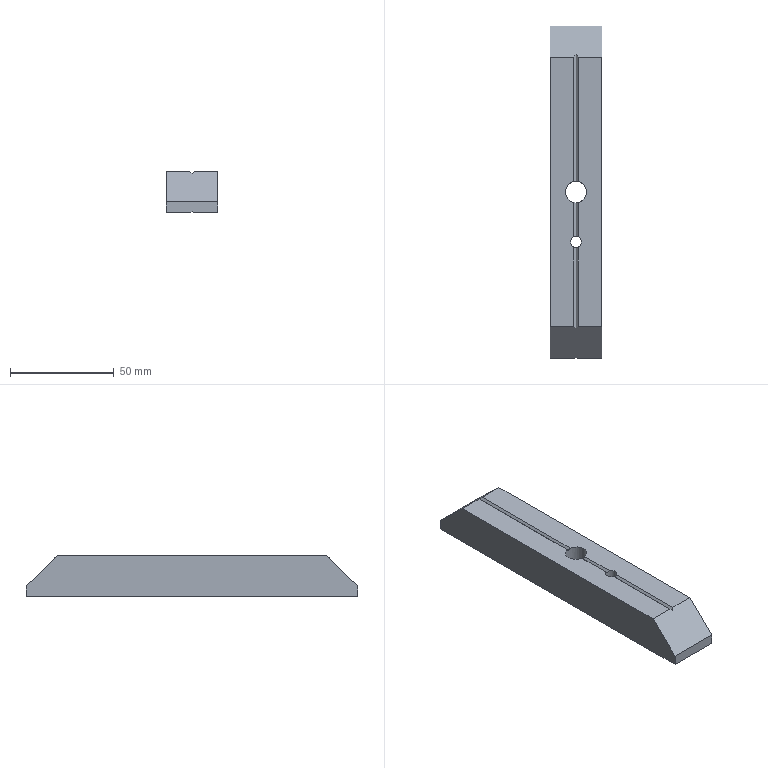Part | NX | features EXTRUDE 3, DATUM_CSYS 1 | 1 solid | 25 faces | box 25 x 160 x 19.5 mm | volume 70356 mm3 | plane 22 | cylinder 2 | spline 1 | commonest cylinder face diameters 5.3 x1 10.3 x1
STEP:
#1=CARTESIAN_POINT('',(3903.536,6799.606,-19.5));
#2=VERTEX_POINT('',#1);
#3=CARTESIAN_POINT('',(3915.536,6799.606,-19.5));
#4=VERTEX_POINT('',#3);
#5=CARTESIAN_POINT('',(3890.536,6799.606,-19.5));
#6=DIRECTION('',(1.,0.,0.));
#7=VECTOR('',#6,1000.);
#8=LINE('',#5,#7);
#9=EDGE_CURVE('',#2,#4,#8,.T.);
#10=ORIENTED_EDGE('',*,*,#9,.F.);
#11=CARTESIAN_POINT('',(3903.536,6853.003,-19.5));
#12=VERTEX_POINT('',#11);
#13=CARTESIAN_POINT('',(3903.536,6978.016,-19.5));
#14=DIRECTION('',(0.,-1.,0.));
#15=VECTOR('',#14,1000.);
#16=LINE('',#13,#15);
#17=EDGE_CURVE('',#2,#12,#16,.F.);
#18=ORIENTED_EDGE('',*,*,#17,.T.);
#19=CARTESIAN_POINT('',(3903.536,6858.208,-19.5));
#20=VERTEX_POINT('',#19);
#21=CARTESIAN_POINT('',(3903.036,6855.606,-19.5));
#22=DIRECTION('',(0.,0.,1.));
#23=DIRECTION('',(1.,0.,0.));
#24=AXIS2_PLACEMENT_3D('',#21,#22,#23);
#25=CIRCLE('',#24,2.65);
#26=EDGE_CURVE('',#12,#20,#25,.T.);
#27=ORIENTED_EDGE('',*,*,#26,.T.);
#28=CARTESIAN_POINT('',(3903.536,6874.48,-19.5));
#29=VERTEX_POINT('',#28);
#30=CARTESIAN_POINT('',(3903.536,6978.016,-19.5));
#31=DIRECTION('',(0.,-1.,0.));
#32=VECTOR('',#31,1000.);
#33=LINE('',#30,#32);
#34=EDGE_CURVE('',#20,#29,#33,.F.);
#35=ORIENTED_EDGE('',*,*,#34,.T.);
#36=CARTESIAN_POINT('',(3903.536,6884.731,-19.5));
#37=VERTEX_POINT('',#36);
#38=CARTESIAN_POINT('',(3903.036,6879.606,-19.5));
#39=DIRECTION('',(0.,0.,1.));
#40=DIRECTION('',(1.,0.,0.));
#41=AXIS2_PLACEMENT_3D('',#38,#39,#40);
#42=CIRCLE('',#41,5.15);
#43=EDGE_CURVE('',#29,#37,#42,.T.);
#44=ORIENTED_EDGE('',*,*,#43,.T.);
#45=CARTESIAN_POINT('',(3903.536,6959.606,-19.5));
#46=VERTEX_POINT('',#45);
#47=CARTESIAN_POINT('',(3903.536,6978.016,-19.5));
#48=DIRECTION('',(0.,-1.,0.));
#49=VECTOR('',#48,1000.);
#50=LINE('',#47,#49);
#51=EDGE_CURVE('',#37,#46,#50,.F.);
#52=ORIENTED_EDGE('',*,*,#51,.T.);
#53=CARTESIAN_POINT('',(3915.536,6959.606,-19.5));
#54=VERTEX_POINT('',#53);
#55=CARTESIAN_POINT('',(3890.536,6959.606,-19.5));
#56=DIRECTION('',(1.,0.,0.));
#57=VECTOR('',#56,1000.);
#58=LINE('',#55,#57);
#59=EDGE_CURVE('',#46,#54,#58,.T.);
#60=ORIENTED_EDGE('',*,*,#59,.T.);
#61=CARTESIAN_POINT('',(3915.536,6959.606,-19.5));
#62=DIRECTION('',(0.,-1.,0.));
#63=VECTOR('',#62,1000.);
#64=LINE('',#61,#63);
#65=EDGE_CURVE('',#54,#4,#64,.T.);
#66=ORIENTED_EDGE('',*,*,#65,.T.);
#67=EDGE_LOOP('',(#10,#18,#27,#35,#44,#52,#60,#66));
#68=FACE_BOUND('',#67,.T.);
#69=CARTESIAN_POINT('',(3890.536,6959.606,-19.5));
#70=DIRECTION('',(0.,0.,1.));
#71=DIRECTION('',(1.,0.,0.));
#72=AXIS2_PLACEMENT_3D('',#69,#70,#71);
#73=PLANE('',#72);
#74=ADVANCED_FACE('',(#68),#73,.F.);
#75=CARTESIAN_POINT('',(3902.536,6858.208,-19.5));
#76=VERTEX_POINT('',#75);
#77=CARTESIAN_POINT('',(3902.536,6853.003,-19.5));
#78=VERTEX_POINT('',#77);
#79=CARTESIAN_POINT('',(3903.036,6855.606,-19.5));
#80=DIRECTION('',(0.,0.,1.));
#81=DIRECTION('',(1.,0.,0.));
#82=AXIS2_PLACEMENT_3D('',#79,#80,#81);
#83=CIRCLE('',#82,2.65);
#84=EDGE_CURVE('',#76,#78,#83,.T.);
#85=ORIENTED_EDGE('',*,*,#84,.T.);
#86=CARTESIAN_POINT('',(3902.536,6799.606,-19.5));
#87=VERTEX_POINT('',#86);
#88=CARTESIAN_POINT('',(3902.536,6978.016,-19.5));
#89=DIRECTION('',(0.,1.,0.));
#90=VECTOR('',#89,1000.);
#91=LINE('',#88,#90);
#92=EDGE_CURVE('',#78,#87,#91,.F.);
#93=ORIENTED_EDGE('',*,*,#92,.T.);
#94=CARTESIAN_POINT('',(3890.536,6799.606,-19.5));
#95=VERTEX_POINT('',#94);
#96=CARTESIAN_POINT('',(3890.536,6799.606,-19.5));
#97=DIRECTION('',(1.,0.,0.));
#98=VECTOR('',#97,1000.);
#99=LINE('',#96,#98);
#100=EDGE_CURVE('',#95,#87,#99,.T.);
#101=ORIENTED_EDGE('',*,*,#100,.F.);
#102=CARTESIAN_POINT('',(3890.536,6959.606,-19.5));
#103=VERTEX_POINT('',#102);
#104=CARTESIAN_POINT('',(3890.536,6959.606,-19.5));
#105=DIRECTION('',(0.,-1.,0.));
#106=VECTOR('',#105,1000.);
#107=LINE('',#104,#106);
#108=EDGE_CURVE('',#103,#95,#107,.T.);
#109=ORIENTED_EDGE('',*,*,#108,.F.);
#110=CARTESIAN_POINT('',(3902.536,6959.606,-19.5));
#111=VERTEX_POINT('',#110);
#112=CARTESIAN_POINT('',(3890.536,6959.606,-19.5));
#113=DIRECTION('',(1.,0.,0.));
#114=VECTOR('',#113,1000.);
#115=LINE('',#112,#114);
#116=EDGE_CURVE('',#103,#111,#115,.T.);
#117=ORIENTED_EDGE('',*,*,#116,.T.);
#118=CARTESIAN_POINT('',(3902.536,6884.731,-19.5));
#119=VERTEX_POINT('',#118);
#120=CARTESIAN_POINT('',(3902.536,6978.016,-19.5));
#121=DIRECTION('',(0.,1.,0.));
#122=VECTOR('',#121,1000.);
#123=LINE('',#120,#122);
#124=EDGE_CURVE('',#111,#119,#123,.F.);
#125=ORIENTED_EDGE('',*,*,#124,.T.);
#126=CARTESIAN_POINT('',(3902.036,6874.554,-19.5));
#127=VERTEX_POINT('',#126);
#128=CARTESIAN_POINT('',(3903.036,6879.606,-19.5));
#129=DIRECTION('',(0.,0.,1.));
#130=DIRECTION('',(1.,0.,0.));
#131=AXIS2_PLACEMENT_3D('',#128,#129,#130);
#132=CIRCLE('',#131,5.15);
#133=EDGE_CURVE('',#119,#127,#132,.T.);
#134=ORIENTED_EDGE('',*,*,#133,.T.);
#135=CARTESIAN_POINT('',(3902.536,6874.48,-19.5));
#136=VERTEX_POINT('',#135);
#137=CARTESIAN_POINT('',(3903.036,6879.606,-19.5));
#138=DIRECTION('',(0.,0.,-1.));
#139=DIRECTION('',(-0.9963,0.0857,0.));
#140=AXIS2_PLACEMENT_3D('',#137,#138,#139);
#141=ELLIPSE('',#140,5.15,5.15);
#142=EDGE_CURVE('',#127,#136,#141,.F.);
#143=ORIENTED_EDGE('',*,*,#142,.T.);
#144=CARTESIAN_POINT('',(3902.536,6978.016,-19.5));
#145=DIRECTION('',(0.,1.,0.));
#146=VECTOR('',#145,1000.);
#147=LINE('',#144,#146);
#148=EDGE_CURVE('',#136,#76,#147,.F.);
#149=ORIENTED_EDGE('',*,*,#148,.T.);
#150=EDGE_LOOP('',(#85,#93,#101,#109,#117,#125,#134,#143,#149));
#151=FACE_BOUND('',#150,.T.);
#152=CARTESIAN_POINT('',(3890.536,6959.606,-19.5));
#153=DIRECTION('',(0.,0.,1.));
#154=DIRECTION('',(1.,0.,0.));
#155=AXIS2_PLACEMENT_3D('',#152,#153,#154);
#156=PLANE('',#155);
#157=ADVANCED_FACE('',(#151),#156,.F.);
#158=CARTESIAN_POINT('',(3904.036,6858.06,0.));
#159=VERTEX_POINT('',#158);
#160=CARTESIAN_POINT('',(3904.036,6853.151,0.));
#161=VERTEX_POINT('',#160);
#162=CARTESIAN_POINT('',(3903.036,6855.606,0.));
#163=DIRECTION('',(0.,0.,-1.));
#164=DIRECTION('',(1.,0.,0.));
#165=AXIS2_PLACEMENT_3D('',#162,#163,#164);
#166=CIRCLE('',#165,2.65);
#167=EDGE_CURVE('',#159,#161,#166,.T.);
#168=ORIENTED_EDGE('',*,*,#167,.T.);
#169=CARTESIAN_POINT('',(3904.036,6814.606,0.));
#170=VERTEX_POINT('',#169);
#171=CARTESIAN_POINT('',(3904.036,6978.016,0.));
#172=DIRECTION('',(0.,1.,0.));
#173=VECTOR('',#172,1000.);
#174=LINE('',#171,#173);
#175=EDGE_CURVE('',#161,#170,#174,.F.);
#176=ORIENTED_EDGE('',*,*,#175,.T.);
#177=CARTESIAN_POINT('',(3915.536,6814.606,0.));
#178=VERTEX_POINT('',#177);
#179=CARTESIAN_POINT('',(3890.536,6814.606,0.));
#180=DIRECTION('',(1.,0.,0.));
#181=VECTOR('',#180,1000.);
#182=LINE('',#179,#181);
#183=EDGE_CURVE('',#170,#178,#182,.T.);
#184=ORIENTED_EDGE('',*,*,#183,.T.);
#185=CARTESIAN_POINT('',(3915.536,6944.606,0.));
#186=VERTEX_POINT('',#185);
#187=CARTESIAN_POINT('',(3915.536,6814.606,0.));
#188=DIRECTION('',(0.,1.,0.));
#189=VECTOR('',#188,1000.);
#190=LINE('',#187,#189);
#191=EDGE_CURVE('',#178,#186,#190,.T.);
#192=ORIENTED_EDGE('',*,*,#191,.T.);
#193=CARTESIAN_POINT('',(3904.036,6944.606,0.));
#194=VERTEX_POINT('',#193);
#195=CARTESIAN_POINT('',(3890.536,6944.606,0.));
#196=DIRECTION('',(1.,0.,0.));
#197=VECTOR('',#196,1000.);
#198=LINE('',#195,#197);
#199=EDGE_CURVE('',#194,#186,#198,.T.);
#200=ORIENTED_EDGE('',*,*,#199,.F.);
#201=CARTESIAN_POINT('',(3904.036,6884.657,0.));
#202=VERTEX_POINT('',#201);
#203=CARTESIAN_POINT('',(3904.036,6978.016,0.));
#204=DIRECTION('',(0.,1.,0.));
#205=VECTOR('',#204,1000.);
#206=LINE('',#203,#205);
#207=EDGE_CURVE('',#194,#202,#206,.F.);
#208=ORIENTED_EDGE('',*,*,#207,.T.);
#209=CARTESIAN_POINT('',(3904.036,6874.554,0.));
#210=VERTEX_POINT('',#209);
#211=CARTESIAN_POINT('',(3903.036,6879.606,0.));
#212=DIRECTION('',(0.,0.,-1.));
#213=DIRECTION('',(1.,0.,0.));
#214=AXIS2_PLACEMENT_3D('',#211,#212,#213);
#215=CIRCLE('',#214,5.15);
#216=EDGE_CURVE('',#202,#210,#215,.T.);
#217=ORIENTED_EDGE('',*,*,#216,.T.);
#218=CARTESIAN_POINT('',(3904.036,6978.016,0.));
#219=DIRECTION('',(0.,1.,0.));
#220=VECTOR('',#219,1000.);
#221=LINE('',#218,#220);
#222=EDGE_CURVE('',#210,#159,#221,.F.);
#223=ORIENTED_EDGE('',*,*,#222,.T.);
#224=EDGE_LOOP('',(#168,#176,#184,#192,#200,#208,#217,#223));
#225=FACE_BOUND('',#224,.T.);
#226=CARTESIAN_POINT('',(3890.536,6814.606,0.));
#227=DIRECTION('',(0.,0.,-1.));
#228=DIRECTION('',(0.,1.,0.));
#229=AXIS2_PLACEMENT_3D('',#226,#227,#228);
#230=PLANE('',#229);
#231=ADVANCED_FACE('',(#225),#230,.F.);
#232=CARTESIAN_POINT('',(3890.536,6814.606,0.));
#233=VERTEX_POINT('',#232);
#234=CARTESIAN_POINT('',(3902.036,6814.606,0.));
#235=VERTEX_POINT('',#234);
#236=CARTESIAN_POINT('',(3890.536,6814.606,0.));
#237=DIRECTION('',(1.,0.,0.));
#238=VECTOR('',#237,1000.);
#239=LINE('',#236,#238);
#240=EDGE_CURVE('',#233,#235,#239,.T.);
#241=ORIENTED_EDGE('',*,*,#240,.T.);
#242=CARTESIAN_POINT('',(3902.036,6853.151,0.));
#243=VERTEX_POINT('',#242);
#244=CARTESIAN_POINT('',(3902.036,6978.016,0.));
#245=DIRECTION('',(0.,-1.,0.));
#246=VECTOR('',#245,1000.);
#247=LINE('',#244,#246);
#248=EDGE_CURVE('',#235,#243,#247,.F.);
#249=ORIENTED_EDGE('',*,*,#248,.T.);
#250=CARTESIAN_POINT('',(3902.036,6858.06,0.));
#251=VERTEX_POINT('',#250);
#252=CARTESIAN_POINT('',(3903.036,6855.606,0.));
#253=DIRECTION('',(0.,0.,-1.));
#254=DIRECTION('',(1.,0.,0.));
#255=AXIS2_PLACEMENT_3D('',#252,#253,#254);
#256=CIRCLE('',#255,2.65);
#257=EDGE_CURVE('',#243,#251,#256,.T.);
#258=ORIENTED_EDGE('',*,*,#257,.T.);
#259=CARTESIAN_POINT('',(3902.036,6874.554,0.));
#260=VERTEX_POINT('',#259);
#261=CARTESIAN_POINT('',(3902.036,6978.016,0.));
#262=DIRECTION('',(0.,-1.,0.));
#263=VECTOR('',#262,1000.);
#264=LINE('',#261,#263);
#265=EDGE_CURVE('',#251,#260,#264,.F.);
#266=ORIENTED_EDGE('',*,*,#265,.T.);
#267=CARTESIAN_POINT('',(3902.036,6884.657,0.));
#268=VERTEX_POINT('',#267);
#269=CARTESIAN_POINT('',(3903.036,6879.606,0.));
#270=DIRECTION('',(0.,0.,-1.));
#271=DIRECTION('',(1.,0.,0.));
#272=AXIS2_PLACEMENT_3D('',#269,#270,#271);
#273=CIRCLE('',#272,5.15);
#274=EDGE_CURVE('',#260,#268,#273,.T.);
#275=ORIENTED_EDGE('',*,*,#274,.T.);
#276=CARTESIAN_POINT('',(3902.036,6944.606,0.));
#277=VERTEX_POINT('',#276);
#278=CARTESIAN_POINT('',(3902.036,6978.016,0.));
#279=DIRECTION('',(0.,-1.,0.));
#280=VECTOR('',#279,1000.);
#281=LINE('',#278,#280);
#282=EDGE_CURVE('',#268,#277,#281,.F.);
#283=ORIENTED_EDGE('',*,*,#282,.T.);
#284=CARTESIAN_POINT('',(3890.536,6944.606,0.));
#285=VERTEX_POINT('',#284);
#286=CARTESIAN_POINT('',(3890.536,6944.606,0.));
#287=DIRECTION('',(1.,0.,0.));
#288=VECTOR('',#287,1000.);
#289=LINE('',#286,#288);
#290=EDGE_CURVE('',#285,#277,#289,.T.);
#291=ORIENTED_EDGE('',*,*,#290,.F.);
#292=CARTESIAN_POINT('',(3890.536,6814.606,0.));
#293=DIRECTION('',(0.,1.,0.));
#294=VECTOR('',#293,1000.);
#295=LINE('',#292,#294);
#296=EDGE_CURVE('',#233,#285,#295,.T.);
#297=ORIENTED_EDGE('',*,*,#296,.F.);
#298=EDGE_LOOP('',(#241,#249,#258,#266,#275,#283,#291,#297));
#299=FACE_BOUND('',#298,.T.);
#300=CARTESIAN_POINT('',(3890.536,6814.606,0.));
#301=DIRECTION('',(0.,0.,-1.));
#302=DIRECTION('',(0.,1.,0.));
#303=AXIS2_PLACEMENT_3D('',#300,#301,#302);
#304=PLANE('',#303);
#305=ADVANCED_FACE('',(#299),#304,.F.);
#306=CARTESIAN_POINT('',(3903.036,6884.756,-1.));
#307=VERTEX_POINT('',#306);
#308=CARTESIAN_POINT('',(3903.036,6879.606,-1.));
#309=DIRECTION('',(0.7071,0.,-0.7071));
#310=DIRECTION('',(0.7071,0.,0.7071));
#311=AXIS2_PLACEMENT_3D('',#308,#309,#310);
#312=ELLIPSE('',#311,7.283,5.15);
#313=EDGE_CURVE('',#202,#307,#312,.F.);
#314=ORIENTED_EDGE('',*,*,#313,.T.);
#315=CARTESIAN_POINT('',(3903.036,6879.606,-1.));
#316=DIRECTION('',(-0.7071,0.,-0.7071));
#317=DIRECTION('',(-0.7071,0.,0.7071));
#318=AXIS2_PLACEMENT_3D('',#315,#316,#317);
#319=ELLIPSE('',#318,7.283,5.15);
#320=EDGE_CURVE('',#307,#268,#319,.F.);
#321=ORIENTED_EDGE('',*,*,#320,.T.);
#322=ORIENTED_EDGE('',*,*,#274,.F.);
#323=CARTESIAN_POINT('',(3902.036,6874.554,-19.5));
#324=CARTESIAN_POINT('',(3902.036,6874.554,-13.));
#325=CARTESIAN_POINT('',(3902.036,6874.554,-6.5));
#326=CARTESIAN_POINT('',(3902.036,6874.554,0.));
#327=B_SPLINE_CURVE_WITH_KNOTS('',3,(#323,#324,#325,#326),.UNSPECIFIED.,.F.,.F.,(4,4),(0.9996,1.),.UNSPECIFIED.);
#328=EDGE_CURVE('',#127,#260,#327,.T.);
#329=ORIENTED_EDGE('',*,*,#328,.F.);
#330=ORIENTED_EDGE('',*,*,#133,.F.);
#331=CARTESIAN_POINT('',(3903.036,6884.756,-19.));
#332=VERTEX_POINT('',#331);
#333=CARTESIAN_POINT('',(3903.036,6879.606,-19.));
#334=DIRECTION('',(-0.7071,0.,0.7071));
#335=DIRECTION('',(0.7071,0.,0.7071));
#336=AXIS2_PLACEMENT_3D('',#333,#334,#335);
#337=ELLIPSE('',#336,7.283,5.15);
#338=EDGE_CURVE('',#119,#332,#337,.F.);
#339=ORIENTED_EDGE('',*,*,#338,.T.);
#340=CARTESIAN_POINT('',(3903.036,6879.606,-19.));
#341=DIRECTION('',(0.7071,0.,0.7071));
#342=DIRECTION('',(-0.7071,0.,0.7071));
#343=AXIS2_PLACEMENT_3D('',#340,#341,#342);
#344=ELLIPSE('',#343,7.283,5.15);
#345=EDGE_CURVE('',#332,#37,#344,.F.);
#346=ORIENTED_EDGE('',*,*,#345,.T.);
#347=ORIENTED_EDGE('',*,*,#43,.F.);
#348=CARTESIAN_POINT('',(3903.036,6874.456,-19.));
#349=VERTEX_POINT('',#348);
#350=CARTESIAN_POINT('',(3903.036,6879.606,-19.));
#351=DIRECTION('',(0.7071,0.,0.7071));
#352=DIRECTION('',(-0.7071,0.,0.7071));
#353=AXIS2_PLACEMENT_3D('',#350,#351,#352);
#354=ELLIPSE('',#353,7.283,5.15);
#355=EDGE_CURVE('',#29,#349,#354,.F.);
#356=ORIENTED_EDGE('',*,*,#355,.T.);
#357=CARTESIAN_POINT('',(3903.036,6874.456,-1.));
#358=VERTEX_POINT('',#357);
#359=CARTESIAN_POINT('',(3903.036,6874.456,-1.));
#360=CARTESIAN_POINT('',(3903.036,6874.456,-7.));
#361=CARTESIAN_POINT('',(3903.036,6874.456,-13.));
#362=CARTESIAN_POINT('',(3903.036,6874.456,-19.));
#363=B_SPLINE_CURVE_WITH_KNOTS('',3,(#359,#360,#361,#362),.UNSPECIFIED.,.F.,.F.,(4,4),(0.00001818,0.0003455),.UNSPECIFIED.);
#364=EDGE_CURVE('',#358,#349,#363,.T.);
#365=ORIENTED_EDGE('',*,*,#364,.F.);
#366=CARTESIAN_POINT('',(3903.036,6879.606,-1.));
#367=DIRECTION('',(0.7071,0.,-0.7071));
#368=DIRECTION('',(0.7071,0.,0.7071));
#369=AXIS2_PLACEMENT_3D('',#366,#367,#368);
#370=ELLIPSE('',#369,7.283,5.15);
#371=EDGE_CURVE('',#358,#210,#370,.F.);
#372=ORIENTED_EDGE('',*,*,#371,.T.);
#373=ORIENTED_EDGE('',*,*,#216,.F.);
#374=EDGE_LOOP('',(#314,#321,#322,#329,#330,#339,#346,#347,#356,#365,#372,#373));
#375=FACE_BOUND('',#374,.T.);
#376=CARTESIAN_POINT('',(3903.036,6879.606,-55000.));
#377=DIRECTION('',(0.,0.,1.));
#378=DIRECTION('',(1.,0.,0.));
#379=AXIS2_PLACEMENT_3D('',#376,#377,#378);
#380=CYLINDRICAL_SURFACE('',#379,5.15);
#381=ADVANCED_FACE('',(#375),#380,.F.);
#382=ORIENTED_EDGE('',*,*,#364,.T.);
#383=CARTESIAN_POINT('',(3903.036,6874.456,-19.));
#384=CARTESIAN_POINT('',(3902.869,6874.456,-19.167));
#385=CARTESIAN_POINT('',(3902.703,6874.464,-19.334));
#386=CARTESIAN_POINT('',(3902.536,6874.48,-19.5));
#387=B_SPLINE_CURVE_WITH_KNOTS('',3,(#383,#384,#385,#386),.UNSPECIFIED.,.F.,.F.,(4,4),(0.,0.0007075),.UNSPECIFIED.);
#388=EDGE_CURVE('',#349,#136,#387,.T.);
#389=ORIENTED_EDGE('',*,*,#388,.T.);
#390=ORIENTED_EDGE('',*,*,#142,.F.);
#391=ORIENTED_EDGE('',*,*,#328,.T.);
#392=CARTESIAN_POINT('',(3902.036,6874.554,-0.00001317));
#393=CARTESIAN_POINT('',(3902.368,6874.488,-0.3317));
#394=CARTESIAN_POINT('',(3902.701,6874.456,-0.6651));
#395=CARTESIAN_POINT('',(3903.036,6874.456,-1.));
#396=B_SPLINE_CURVE_WITH_KNOTS('',3,(#392,#393,#394,#395),.UNSPECIFIED.,.F.,.F.,(4,4),(0.,0.001418),.UNSPECIFIED.);
#397=EDGE_CURVE('',#260,#358,#396,.T.);
#398=ORIENTED_EDGE('',*,*,#397,.T.);
#399=EDGE_LOOP('',(#382,#389,#390,#391,#398));
#400=FACE_BOUND('',#399,.T.);
#401=CARTESIAN_POINT('',(3903.036,6874.456,-19.5));
#402=CARTESIAN_POINT('',(3903.036,6874.456,0.117));
#403=CARTESIAN_POINT('',(3902.701,6874.456,-19.5));
#404=CARTESIAN_POINT('',(3902.701,6874.456,0.117));
#405=CARTESIAN_POINT('',(3902.365,6874.488,-19.5));
#406=CARTESIAN_POINT('',(3902.365,6874.488,0.117));
#407=CARTESIAN_POINT('',(3902.036,6874.554,-19.5));
#408=CARTESIAN_POINT('',(3902.036,6874.554,0.117));
#409=B_SPLINE_SURFACE_WITH_KNOTS('',3,1,((#401,#402),(#403,#404),(#405,#406),(#407,#408)),.SURF_OF_LINEAR_EXTRUSION.,.F.,.F.,.F.,(4,4),(2,2),(4.627,4.822),(0.,1.),.PIECEWISE_BEZIER_KNOTS.);
#410=ADVANCED_FACE('',(#400),#409,.T.);
#411=ORIENTED_EDGE('',*,*,#26,.F.);
#412=CARTESIAN_POINT('',(3903.036,6852.956,-19.));
#413=VERTEX_POINT('',#412);
#414=CARTESIAN_POINT('',(3903.036,6855.606,-19.));
#415=DIRECTION('',(0.7071,0.,0.7071));
#416=DIRECTION('',(-0.7071,0.,0.7071));
#417=AXIS2_PLACEMENT_3D('',#414,#415,#416);
#418=ELLIPSE('',#417,3.748,2.65);
#419=EDGE_CURVE('',#12,#413,#418,.F.);
#420=ORIENTED_EDGE('',*,*,#419,.T.);
#421=CARTESIAN_POINT('',(3903.036,6855.606,-19.));
#422=DIRECTION('',(-0.7071,0.,0.7071));
#423=DIRECTION('',(0.7071,0.,0.7071));
#424=AXIS2_PLACEMENT_3D('',#421,#422,#423);
#425=ELLIPSE('',#424,3.748,2.65);
#426=EDGE_CURVE('',#413,#78,#425,.F.);
#427=ORIENTED_EDGE('',*,*,#426,.T.);
#428=ORIENTED_EDGE('',*,*,#84,.F.);
#429=CARTESIAN_POINT('',(3903.036,6858.256,-19.));
#430=VERTEX_POINT('',#429);
#431=CARTESIAN_POINT('',(3903.036,6855.606,-19.));
#432=DIRECTION('',(-0.7071,0.,0.7071));
#433=DIRECTION('',(0.7071,0.,0.7071));
#434=AXIS2_PLACEMENT_3D('',#431,#432,#433);
#435=ELLIPSE('',#434,3.748,2.65);
#436=EDGE_CURVE('',#76,#430,#435,.F.);
#437=ORIENTED_EDGE('',*,*,#436,.T.);
#438=CARTESIAN_POINT('',(3903.036,6855.606,-19.));
#439=DIRECTION('',(0.7071,0.,0.7071));
#440=DIRECTION('',(-0.7071,0.,0.7071));
#441=AXIS2_PLACEMENT_3D('',#438,#439,#440);
#442=ELLIPSE('',#441,3.748,2.65);
#443=EDGE_CURVE('',#430,#20,#442,.F.);
#444=ORIENTED_EDGE('',*,*,#443,.T.);
#445=EDGE_LOOP('',(#411,#420,#427,#428,#437,#444));
#446=FACE_BOUND('',#445,.T.);
#447=ORIENTED_EDGE('',*,*,#257,.F.);
#448=CARTESIAN_POINT('',(3903.036,6852.956,-1.));
#449=VERTEX_POINT('',#448);
#450=CARTESIAN_POINT('',(3903.036,6855.606,-1.));
#451=DIRECTION('',(-0.7071,0.,-0.7071));
#452=DIRECTION('',(-0.7071,0.,0.7071));
#453=AXIS2_PLACEMENT_3D('',#450,#451,#452);
#454=ELLIPSE('',#453,3.748,2.65);
#455=EDGE_CURVE('',#243,#449,#454,.F.);
#456=ORIENTED_EDGE('',*,*,#455,.T.);
#457=CARTESIAN_POINT('',(3903.036,6855.606,-1.));
#458=DIRECTION('',(0.7071,0.,-0.7071));
#459=DIRECTION('',(0.7071,0.,0.7071));
#460=AXIS2_PLACEMENT_3D('',#457,#458,#459);
#461=ELLIPSE('',#460,3.748,2.65);
#462=EDGE_CURVE('',#449,#161,#461,.F.);
#463=ORIENTED_EDGE('',*,*,#462,.T.);
#464=ORIENTED_EDGE('',*,*,#167,.F.);
#465=CARTESIAN_POINT('',(3903.036,6858.256,-1.));
#466=VERTEX_POINT('',#465);
#467=CARTESIAN_POINT('',(3903.036,6855.606,-1.));
#468=DIRECTION('',(0.7071,0.,-0.7071));
#469=DIRECTION('',(0.7071,0.,0.7071));
#470=AXIS2_PLACEMENT_3D('',#467,#468,#469);
#471=ELLIPSE('',#470,3.748,2.65);
#472=EDGE_CURVE('',#159,#466,#471,.F.);
#473=ORIENTED_EDGE('',*,*,#472,.T.);
#474=CARTESIAN_POINT('',(3903.036,6855.606,-1.));
#475=DIRECTION('',(-0.7071,0.,-0.7071));
#476=DIRECTION('',(-0.7071,0.,0.7071));
#477=AXIS2_PLACEMENT_3D('',#474,#475,#476);
#478=ELLIPSE('',#477,3.748,2.65);
#479=EDGE_CURVE('',#466,#251,#478,.F.);
#480=ORIENTED_EDGE('',*,*,#479,.T.);
#481=EDGE_LOOP('',(#447,#456,#463,#464,#473,#480));
#482=FACE_BOUND('',#481,.T.);
#483=CARTESIAN_POINT('',(3903.036,6855.606,-55000.));
#484=DIRECTION('',(0.,0.,1.));
#485=DIRECTION('',(1.,0.,0.));
#486=AXIS2_PLACEMENT_3D('',#483,#484,#485);
#487=CYLINDRICAL_SURFACE('',#486,2.65);
#488=ADVANCED_FACE('',(#446,#482),#487,.F.);
#489=CARTESIAN_POINT('',(3903.036,6959.606,-19.));
#490=VERTEX_POINT('',#489);
#491=CARTESIAN_POINT('',(3904.036,6959.606,-20.));
#492=DIRECTION('',(0.7071,0.,-0.7071));
#493=VECTOR('',#492,1000.);
#494=LINE('',#491,#493);
#495=EDGE_CURVE('',#46,#490,#494,.F.);
#496=ORIENTED_EDGE('',*,*,#495,.T.);
#497=CARTESIAN_POINT('',(3903.036,6959.606,-19.));
#498=DIRECTION('',(0.7071,0.,0.7071));
#499=VECTOR('',#498,1000.);
#500=LINE('',#497,#499);
#501=EDGE_CURVE('',#490,#111,#500,.F.);
#502=ORIENTED_EDGE('',*,*,#501,.T.);
#503=ORIENTED_EDGE('',*,*,#116,.F.);
#504=CARTESIAN_POINT('',(3890.536,6959.606,-14.5));
#505=VERTEX_POINT('',#504);
#506=CARTESIAN_POINT('',(3890.536,6959.606,-14.5));
#507=DIRECTION('',(0.,0.,-1.));
#508=VECTOR('',#507,1000.);
#509=LINE('',#506,#508);
#510=EDGE_CURVE('',#505,#103,#509,.T.);
#511=ORIENTED_EDGE('',*,*,#510,.F.);
#512=CARTESIAN_POINT('',(3915.536,6959.606,-14.5));
#513=VERTEX_POINT('',#512);
#514=CARTESIAN_POINT('',(3890.536,6959.606,-14.5));
#515=DIRECTION('',(1.,0.,0.));
#516=VECTOR('',#515,1000.);
#517=LINE('',#514,#516);
#518=EDGE_CURVE('',#505,#513,#517,.T.);
#519=ORIENTED_EDGE('',*,*,#518,.T.);
#520=CARTESIAN_POINT('',(3915.536,6959.606,-14.5));
#521=DIRECTION('',(0.,0.,-1.));
#522=VECTOR('',#521,1000.);
#523=LINE('',#520,#522);
#524=EDGE_CURVE('',#513,#54,#523,.T.);
#525=ORIENTED_EDGE('',*,*,#524,.T.);
#526=ORIENTED_EDGE('',*,*,#59,.F.);
#527=EDGE_LOOP('',(#496,#502,#503,#511,#519,#525,#526));
#528=FACE_BOUND('',#527,.T.);
#529=CARTESIAN_POINT('',(3890.536,6959.606,-14.5));
#530=DIRECTION('',(0.,-1.,0.));
#531=DIRECTION('',(0.,0.,-1.));
#532=AXIS2_PLACEMENT_3D('',#529,#530,#531);
#533=PLANE('',#532);
#534=ADVANCED_FACE('',(#528),#533,.F.);
#535=CARTESIAN_POINT('',(3903.036,6799.606,-19.));
#536=VERTEX_POINT('',#535);
#537=CARTESIAN_POINT('',(3903.036,6799.606,-19.));
#538=DIRECTION('',(-0.7071,0.,-0.7071));
#539=VECTOR('',#538,1000.);
#540=LINE('',#537,#539);
#541=EDGE_CURVE('',#87,#536,#540,.F.);
#542=ORIENTED_EDGE('',*,*,#541,.T.);
#543=CARTESIAN_POINT('',(3904.036,6799.606,-20.));
#544=DIRECTION('',(-0.7071,0.,0.7071));
#545=VECTOR('',#544,1000.);
#546=LINE('',#543,#545);
#547=EDGE_CURVE('',#536,#2,#546,.F.);
#548=ORIENTED_EDGE('',*,*,#547,.T.);
#549=ORIENTED_EDGE('',*,*,#9,.T.);
#550=CARTESIAN_POINT('',(3915.536,6799.606,-14.5));
#551=VERTEX_POINT('',#550);
#552=CARTESIAN_POINT('',(3915.536,6799.606,-19.5));
#553=DIRECTION('',(0.,0.,1.));
#554=VECTOR('',#553,1000.);
#555=LINE('',#552,#554);
#556=EDGE_CURVE('',#4,#551,#555,.T.);
#557=ORIENTED_EDGE('',*,*,#556,.T.);
#558=CARTESIAN_POINT('',(3890.536,6799.606,-14.5));
#559=VERTEX_POINT('',#558);
#560=CARTESIAN_POINT('',(3890.536,6799.606,-14.5));
#561=DIRECTION('',(1.,0.,0.));
#562=VECTOR('',#561,1000.);
#563=LINE('',#560,#562);
#564=EDGE_CURVE('',#559,#551,#563,.T.);
#565=ORIENTED_EDGE('',*,*,#564,.F.);
#566=CARTESIAN_POINT('',(3890.536,6799.606,-19.5));
#567=DIRECTION('',(0.,0.,1.));
#568=VECTOR('',#567,1000.);
#569=LINE('',#566,#568);
#570=EDGE_CURVE('',#95,#559,#569,.T.);
#571=ORIENTED_EDGE('',*,*,#570,.F.);
#572=ORIENTED_EDGE('',*,*,#100,.T.);
#573=EDGE_LOOP('',(#542,#548,#549,#557,#565,#571,#572));
#574=FACE_BOUND('',#573,.T.);
#575=CARTESIAN_POINT('',(3890.536,6799.606,-19.5));
#576=DIRECTION('',(0.,1.,0.));
#577=DIRECTION('',(0.,0.,1.));
#578=AXIS2_PLACEMENT_3D('',#575,#576,#577);
#579=PLANE('',#578);
#580=ADVANCED_FACE('',(#574),#579,.F.);
#581=CARTESIAN_POINT('',(3903.036,6813.571,-1.));
#582=VERTEX_POINT('',#581);
#583=CARTESIAN_POINT('',(3958.445,6870.891,54.409));
#584=DIRECTION('',(0.5707,0.5904,0.5707));
#585=VECTOR('',#584,1000.);
#586=LINE('',#583,#585);
#587=EDGE_CURVE('',#170,#582,#586,.F.);
#588=ORIENTED_EDGE('',*,*,#587,.T.);
#589=CARTESIAN_POINT('',(3846.975,6871.565,55.061));
#590=DIRECTION('',(0.5707,-0.5904,-0.5707));
#591=VECTOR('',#590,1000.);
#592=LINE('',#589,#591);
#593=EDGE_CURVE('',#582,#235,#592,.F.);
#594=ORIENTED_EDGE('',*,*,#593,.T.);
#595=ORIENTED_EDGE('',*,*,#240,.F.);
#596=CARTESIAN_POINT('',(3890.536,6799.606,-14.5));
#597=DIRECTION('',(0.,0.719,0.695));
#598=VECTOR('',#597,1000.);
#599=LINE('',#596,#598);
#600=EDGE_CURVE('',#559,#233,#599,.T.);
#601=ORIENTED_EDGE('',*,*,#600,.F.);
#602=ORIENTED_EDGE('',*,*,#564,.T.);
#603=CARTESIAN_POINT('',(3915.536,6799.606,-14.5));
#604=DIRECTION('',(0.,0.719,0.695));
#605=VECTOR('',#604,1000.);
#606=LINE('',#603,#605);
#607=EDGE_CURVE('',#551,#178,#606,.T.);
#608=ORIENTED_EDGE('',*,*,#607,.T.);
#609=ORIENTED_EDGE('',*,*,#183,.F.);
#610=EDGE_LOOP('',(#588,#594,#595,#601,#602,#608,#609));
#611=FACE_BOUND('',#610,.T.);
#612=CARTESIAN_POINT('',(3890.536,6799.606,-14.5));
#613=DIRECTION('',(0.,0.695,-0.719));
#614=DIRECTION('',(0.,0.719,0.695));
#615=AXIS2_PLACEMENT_3D('',#612,#613,#614);
#616=PLANE('',#615);
#617=ADVANCED_FACE('',(#611),#616,.F.);
#618=CARTESIAN_POINT('',(3903.036,6945.64,-1.));
#619=VERTEX_POINT('',#618);
#620=CARTESIAN_POINT('',(3913.294,6956.251,-11.257));
#621=DIRECTION('',(-0.5707,-0.5904,0.5707));
#622=VECTOR('',#621,1000.);
#623=LINE('',#620,#622);
#624=EDGE_CURVE('',#277,#619,#623,.F.);
#625=ORIENTED_EDGE('',*,*,#624,.T.);
#626=CARTESIAN_POINT('',(3892.127,6956.925,-11.909));
#627=DIRECTION('',(-0.5707,0.5904,-0.5707));
#628=VECTOR('',#627,1000.);
#629=LINE('',#626,#628);
#630=EDGE_CURVE('',#619,#194,#629,.F.);
#631=ORIENTED_EDGE('',*,*,#630,.T.);
#632=ORIENTED_EDGE('',*,*,#199,.T.);
#633=CARTESIAN_POINT('',(3915.536,6944.606,0.));
#634=DIRECTION('',(0.,0.719,-0.695));
#635=VECTOR('',#634,1000.);
#636=LINE('',#633,#635);
#637=EDGE_CURVE('',#186,#513,#636,.T.);
#638=ORIENTED_EDGE('',*,*,#637,.T.);
#639=ORIENTED_EDGE('',*,*,#518,.F.);
#640=CARTESIAN_POINT('',(3890.536,6944.606,0.));
#641=DIRECTION('',(0.,0.719,-0.695));
#642=VECTOR('',#641,1000.);
#643=LINE('',#640,#642);
#644=EDGE_CURVE('',#285,#505,#643,.T.);
#645=ORIENTED_EDGE('',*,*,#644,.F.);
#646=ORIENTED_EDGE('',*,*,#290,.T.);
#647=EDGE_LOOP('',(#625,#631,#632,#638,#639,#645,#646));
#648=FACE_BOUND('',#647,.T.);
#649=CARTESIAN_POINT('',(3890.536,6944.606,0.));
#650=DIRECTION('',(0.,-0.695,-0.719));
#651=DIRECTION('',(0.,0.719,-0.695));
#652=AXIS2_PLACEMENT_3D('',#649,#650,#651);
#653=PLANE('',#652);
#654=ADVANCED_FACE('',(#648),#653,.F.);
#655=ORIENTED_EDGE('',*,*,#510,.T.);
#656=ORIENTED_EDGE('',*,*,#108,.T.);
#657=ORIENTED_EDGE('',*,*,#570,.T.);
#658=ORIENTED_EDGE('',*,*,#600,.T.);
#659=ORIENTED_EDGE('',*,*,#296,.T.);
#660=ORIENTED_EDGE('',*,*,#644,.T.);
#661=EDGE_LOOP('',(#655,#656,#657,#658,#659,#660));
#662=FACE_BOUND('',#661,.T.);
#663=CARTESIAN_POINT('',(3890.536,0.,0.));
#664=DIRECTION('',(-1.,0.,0.));
#665=DIRECTION('',(0.,0.,1.));
#666=AXIS2_PLACEMENT_3D('',#663,#664,#665);
#667=PLANE('',#666);
#668=ADVANCED_FACE('',(#662),#667,.T.);
#669=ORIENTED_EDGE('',*,*,#524,.F.);
#670=ORIENTED_EDGE('',*,*,#637,.F.);
#671=ORIENTED_EDGE('',*,*,#191,.F.);
#672=ORIENTED_EDGE('',*,*,#607,.F.);
#673=ORIENTED_EDGE('',*,*,#556,.F.);
#674=ORIENTED_EDGE('',*,*,#65,.F.);
#675=EDGE_LOOP('',(#669,#670,#671,#672,#673,#674));
#676=FACE_BOUND('',#675,.T.);
#677=CARTESIAN_POINT('',(3915.536,0.,0.));
#678=DIRECTION('',(-1.,0.,0.));
#679=DIRECTION('',(0.,0.,1.));
#680=AXIS2_PLACEMENT_3D('',#677,#678,#679);
#681=PLANE('',#680);
#682=ADVANCED_FACE('',(#676),#681,.F.);
#683=CARTESIAN_POINT('',(3903.036,6978.016,-1.));
#684=DIRECTION('',(0.,-1.,0.));
#685=VECTOR('',#684,1000.);
#686=LINE('',#683,#685);
#687=EDGE_CURVE('',#466,#358,#686,.F.);
#688=ORIENTED_EDGE('',*,*,#687,.T.);
#689=ORIENTED_EDGE('',*,*,#397,.F.);
#690=ORIENTED_EDGE('',*,*,#265,.F.);
#691=ORIENTED_EDGE('',*,*,#479,.F.);
#692=EDGE_LOOP('',(#688,#689,#690,#691));
#693=FACE_BOUND('',#692,.T.);
#694=CARTESIAN_POINT('',(3902.036,6978.016,0.));
#695=DIRECTION('',(-0.7071,0.,-0.7071));
#696=DIRECTION('',(-0.7071,0.,0.7071));
#697=AXIS2_PLACEMENT_3D('',#694,#695,#696);
#698=PLANE('',#697);
#699=ADVANCED_FACE('',(#693),#698,.F.);
#700=ORIENTED_EDGE('',*,*,#222,.F.);
#701=ORIENTED_EDGE('',*,*,#371,.F.);
#702=ORIENTED_EDGE('',*,*,#687,.F.);
#703=ORIENTED_EDGE('',*,*,#472,.F.);
#704=EDGE_LOOP('',(#700,#701,#702,#703));
#705=FACE_BOUND('',#704,.T.);
#706=CARTESIAN_POINT('',(3903.036,6978.016,-1.));
#707=DIRECTION('',(0.7071,0.,-0.7071));
#708=DIRECTION('',(-0.7071,0.,-0.7071));
#709=AXIS2_PLACEMENT_3D('',#706,#707,#708);
#710=PLANE('',#709);
#711=ADVANCED_FACE('',(#705),#710,.F.);
#712=CARTESIAN_POINT('',(3903.036,6978.016,-19.));
#713=DIRECTION('',(0.,-1.,0.));
#714=VECTOR('',#713,1000.);
#715=LINE('',#712,#714);
#716=EDGE_CURVE('',#430,#349,#715,.F.);
#717=ORIENTED_EDGE('',*,*,#716,.T.);
#718=ORIENTED_EDGE('',*,*,#355,.F.);
#719=ORIENTED_EDGE('',*,*,#34,.F.);
#720=ORIENTED_EDGE('',*,*,#443,.F.);
#721=EDGE_LOOP('',(#717,#718,#719,#720));
#722=FACE_BOUND('',#721,.T.);
#723=CARTESIAN_POINT('',(3904.036,6978.016,-20.));
#724=DIRECTION('',(0.7071,0.,0.7071));
#725=DIRECTION('',(0.7071,0.,-0.7071));
#726=AXIS2_PLACEMENT_3D('',#723,#724,#725);
#727=PLANE('',#726);
#728=ADVANCED_FACE('',(#722),#727,.F.);
#729=ORIENTED_EDGE('',*,*,#148,.F.);
#730=ORIENTED_EDGE('',*,*,#388,.F.);
#731=ORIENTED_EDGE('',*,*,#716,.F.);
#732=ORIENTED_EDGE('',*,*,#436,.F.);
#733=EDGE_LOOP('',(#729,#730,#731,#732));
#734=FACE_BOUND('',#733,.T.);
#735=CARTESIAN_POINT('',(3903.036,6978.016,-19.));
#736=DIRECTION('',(-0.7071,0.,0.7071));
#737=DIRECTION('',(0.7071,0.,0.7071));
#738=AXIS2_PLACEMENT_3D('',#735,#736,#737);
#739=PLANE('',#738);
#740=ADVANCED_FACE('',(#734),#739,.F.);
#741=ORIENTED_EDGE('',*,*,#17,.F.);
#742=ORIENTED_EDGE('',*,*,#547,.F.);
#743=CARTESIAN_POINT('',(3903.036,6978.016,-19.));
#744=DIRECTION('',(0.,-1.,0.));
#745=VECTOR('',#744,1000.);
#746=LINE('',#743,#745);
#747=EDGE_CURVE('',#536,#413,#746,.F.);
#748=ORIENTED_EDGE('',*,*,#747,.T.);
#749=ORIENTED_EDGE('',*,*,#419,.F.);
#750=EDGE_LOOP('',(#741,#742,#748,#749));
#751=FACE_BOUND('',#750,.T.);
#752=CARTESIAN_POINT('',(3904.036,6978.016,-20.));
#753=DIRECTION('',(0.7071,0.,0.7071));
#754=DIRECTION('',(0.7071,0.,-0.7071));
#755=AXIS2_PLACEMENT_3D('',#752,#753,#754);
#756=PLANE('',#755);
#757=ADVANCED_FACE('',(#751),#756,.F.);
#758=ORIENTED_EDGE('',*,*,#747,.F.);
#759=ORIENTED_EDGE('',*,*,#541,.F.);
#760=ORIENTED_EDGE('',*,*,#92,.F.);
#761=ORIENTED_EDGE('',*,*,#426,.F.);
#762=EDGE_LOOP('',(#758,#759,#760,#761));
#763=FACE_BOUND('',#762,.T.);
#764=CARTESIAN_POINT('',(3903.036,6978.016,-19.));
#765=DIRECTION('',(-0.7071,0.,0.7071));
#766=DIRECTION('',(0.7071,0.,0.7071));
#767=AXIS2_PLACEMENT_3D('',#764,#765,#766);
#768=PLANE('',#767);
#769=ADVANCED_FACE('',(#763),#768,.F.);
#770=ORIENTED_EDGE('',*,*,#248,.F.);
#771=ORIENTED_EDGE('',*,*,#593,.F.);
#772=CARTESIAN_POINT('',(3903.036,6978.016,-1.));
#773=DIRECTION('',(0.,-1.,0.));
#774=VECTOR('',#773,1000.);
#775=LINE('',#772,#774);
#776=EDGE_CURVE('',#582,#449,#775,.F.);
#777=ORIENTED_EDGE('',*,*,#776,.T.);
#778=ORIENTED_EDGE('',*,*,#455,.F.);
#779=EDGE_LOOP('',(#770,#771,#777,#778));
#780=FACE_BOUND('',#779,.T.);
#781=CARTESIAN_POINT('',(3902.036,6978.016,0.));
#782=DIRECTION('',(-0.7071,0.,-0.7071));
#783=DIRECTION('',(-0.7071,0.,0.7071));
#784=AXIS2_PLACEMENT_3D('',#781,#782,#783);
#785=PLANE('',#784);
#786=ADVANCED_FACE('',(#780),#785,.F.);
#787=ORIENTED_EDGE('',*,*,#776,.F.);
#788=ORIENTED_EDGE('',*,*,#587,.F.);
#789=ORIENTED_EDGE('',*,*,#175,.F.);
#790=ORIENTED_EDGE('',*,*,#462,.F.);
#791=EDGE_LOOP('',(#787,#788,#789,#790));
#792=FACE_BOUND('',#791,.T.);
#793=CARTESIAN_POINT('',(3903.036,6978.016,-1.));
#794=DIRECTION('',(0.7071,0.,-0.7071));
#795=DIRECTION('',(-0.7071,0.,-0.7071));
#796=AXIS2_PLACEMENT_3D('',#793,#794,#795);
#797=PLANE('',#796);
#798=ADVANCED_FACE('',(#792),#797,.F.);
#799=CARTESIAN_POINT('',(3903.036,6978.016,-19.));
#800=DIRECTION('',(0.,-1.,0.));
#801=VECTOR('',#800,1000.);
#802=LINE('',#799,#801);
#803=EDGE_CURVE('',#332,#490,#802,.F.);
#804=ORIENTED_EDGE('',*,*,#803,.T.);
#805=ORIENTED_EDGE('',*,*,#495,.F.);
#806=ORIENTED_EDGE('',*,*,#51,.F.);
#807=ORIENTED_EDGE('',*,*,#345,.F.);
#808=EDGE_LOOP('',(#804,#805,#806,#807));
#809=FACE_BOUND('',#808,.T.);
#810=CARTESIAN_POINT('',(3904.036,6978.016,-20.));
#811=DIRECTION('',(0.7071,0.,0.7071));
#812=DIRECTION('',(0.7071,0.,-0.7071));
#813=AXIS2_PLACEMENT_3D('',#810,#811,#812);
#814=PLANE('',#813);
#815=ADVANCED_FACE('',(#809),#814,.F.);
#816=ORIENTED_EDGE('',*,*,#124,.F.);
#817=ORIENTED_EDGE('',*,*,#501,.F.);
#818=ORIENTED_EDGE('',*,*,#803,.F.);
#819=ORIENTED_EDGE('',*,*,#338,.F.);
#820=EDGE_LOOP('',(#816,#817,#818,#819));
#821=FACE_BOUND('',#820,.T.);
#822=CARTESIAN_POINT('',(3903.036,6978.016,-19.));
#823=DIRECTION('',(-0.7071,0.,0.7071));
#824=DIRECTION('',(0.7071,0.,0.7071));
#825=AXIS2_PLACEMENT_3D('',#822,#823,#824);
#826=PLANE('',#825);
#827=ADVANCED_FACE('',(#821),#826,.F.);
#828=CARTESIAN_POINT('',(3903.036,6978.016,-1.));
#829=DIRECTION('',(0.,-1.,0.));
#830=VECTOR('',#829,1000.);
#831=LINE('',#828,#830);
#832=EDGE_CURVE('',#307,#619,#831,.F.);
#833=ORIENTED_EDGE('',*,*,#832,.T.);
#834=ORIENTED_EDGE('',*,*,#624,.F.);
#835=ORIENTED_EDGE('',*,*,#282,.F.);
#836=ORIENTED_EDGE('',*,*,#320,.F.);
#837=EDGE_LOOP('',(#833,#834,#835,#836));
#838=FACE_BOUND('',#837,.T.);
#839=CARTESIAN_POINT('',(3902.036,6978.016,0.));
#840=DIRECTION('',(-0.7071,0.,-0.7071));
#841=DIRECTION('',(-0.7071,0.,0.7071));
#842=AXIS2_PLACEMENT_3D('',#839,#840,#841);
#843=PLANE('',#842);
#844=ADVANCED_FACE('',(#838),#843,.F.);
#845=ORIENTED_EDGE('',*,*,#207,.F.);
#846=ORIENTED_EDGE('',*,*,#630,.F.);
#847=ORIENTED_EDGE('',*,*,#832,.F.);
#848=ORIENTED_EDGE('',*,*,#313,.F.);
#849=EDGE_LOOP('',(#845,#846,#847,#848));
#850=FACE_BOUND('',#849,.T.);
#851=CARTESIAN_POINT('',(3903.036,6978.016,-1.));
#852=DIRECTION('',(0.7071,0.,-0.7071));
#853=DIRECTION('',(-0.7071,0.,-0.7071));
#854=AXIS2_PLACEMENT_3D('',#851,#852,#853);
#855=PLANE('',#854);
#856=ADVANCED_FACE('',(#850),#855,.F.);
#857=CLOSED_SHELL('',(#74,#157,#231,#305,#381,#410,#488,#534,#580,#617,#654,#668,#682,#699,#711,#728,#740,#757,#769,#786,#798,#815,#827,#844,#856));
#858=MANIFOLD_SOLID_BREP('',#857);
#859=(LENGTH_UNIT()NAMED_UNIT(*)SI_UNIT(.MILLI.,.METRE.));
#860=UNCERTAINTY_MEASURE_WITH_UNIT(LENGTH_MEASURE(0.0508),#859,'','');
#861=(NAMED_UNIT(*)PLANE_ANGLE_UNIT()SI_UNIT($,.RADIAN.));
#862=(NAMED_UNIT(*)SI_UNIT($,.STERADIAN.)SOLID_ANGLE_UNIT());
#863=(GEOMETRIC_REPRESENTATION_CONTEXT(3)GLOBAL_UNCERTAINTY_ASSIGNED_CONTEXT((#860))GLOBAL_UNIT_ASSIGNED_CONTEXT((#859,#861,#862))REPRESENTATION_CONTEXT('',''));
#864=ADVANCED_BREP_SHAPE_REPRESENTATION('',(#858),#863);